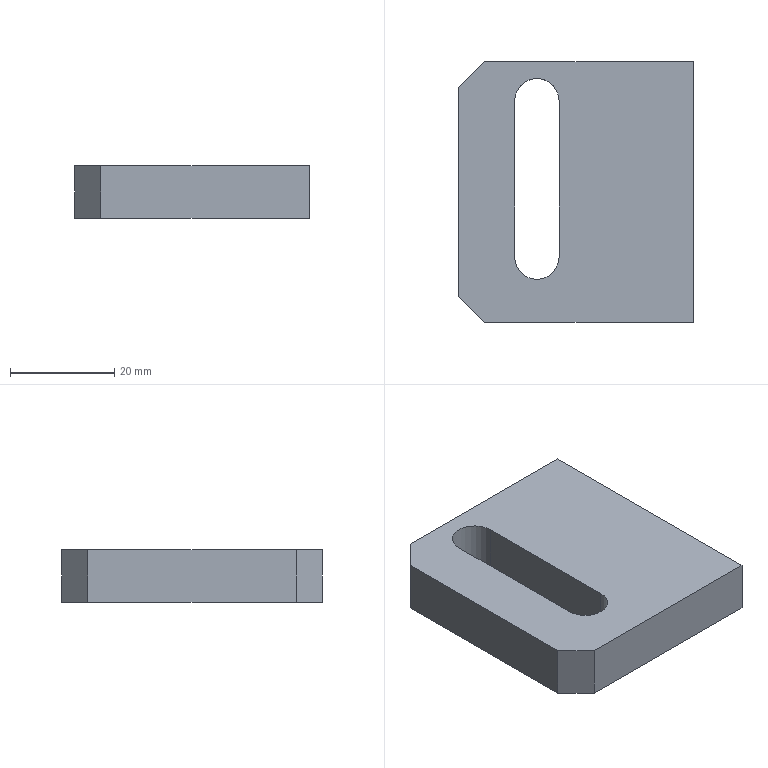Part | SolidWorks | features Chamfer 1, Extrusion 1, HoleWzd 1, ICE 1 | 1 solid | 20 faces | box 45 x 50 x 10 mm | volume 18367 mm3 | plane 10 | cylinder 6 | cone 4 | commonest cylinder face diameters 5 x4 8.5 x2
STEP:
#1=CARTESIAN_POINT('',(-6.787,32.842,7.5));
#2=VERTEX_POINT('',#1);
#3=CARTESIAN_POINT('',(-6.787,32.842,2.5));
#4=VERTEX_POINT('',#3);
#5=CARTESIAN_POINT('',(-6.787,32.842,5.));
#6=DIRECTION('',(1.,0.,0.));
#7=DIRECTION('',(0.,0.,-1.));
#8=AXIS2_PLACEMENT_3D('',#5,#6,#7);
#9=CIRCLE('',#8,2.5);
#10=EDGE_CURVE('',#2,#4,#9,.T.);
#11=ORIENTED_EDGE('',*,*,#10,.F.);
#12=CARTESIAN_POINT('',(12.213,32.842,7.5));
#13=VERTEX_POINT('',#12);
#14=CARTESIAN_POINT('',(12.213,32.842,7.5));
#15=DIRECTION('',(1.,0.,0.));
#16=VECTOR('',#15,1000.);
#17=LINE('',#14,#16);
#18=EDGE_CURVE('',#2,#13,#17,.T.);
#19=ORIENTED_EDGE('',*,*,#18,.T.);
#20=CARTESIAN_POINT('',(12.213,32.842,2.5));
#21=VERTEX_POINT('',#20);
#22=CARTESIAN_POINT('',(12.213,32.842,5.));
#23=DIRECTION('',(1.,0.,0.));
#24=DIRECTION('',(0.,0.,-1.));
#25=AXIS2_PLACEMENT_3D('',#22,#23,#24);
#26=CIRCLE('',#25,2.5);
#27=EDGE_CURVE('',#13,#21,#26,.T.);
#28=ORIENTED_EDGE('',*,*,#27,.T.);
#29=CARTESIAN_POINT('',(12.213,32.842,2.5));
#30=DIRECTION('',(1.,0.,0.));
#31=VECTOR('',#30,1000.);
#32=LINE('',#29,#31);
#33=EDGE_CURVE('',#4,#21,#32,.T.);
#34=ORIENTED_EDGE('',*,*,#33,.F.);
#35=EDGE_LOOP('',(#11,#19,#28,#34));
#36=FACE_OUTER_BOUND('',#35,.T.);
#37=CARTESIAN_POINT('',(12.213,32.842,5.));
#38=DIRECTION('',(1.,0.,0.));
#39=DIRECTION('',(0.,0.,-1.));
#40=AXIS2_PLACEMENT_3D('',#37,#38,#39);
#41=CYLINDRICAL_SURFACE('',#40,2.5);
#42=ADVANCED_FACE('',(#36),#41,.F.);
#43=CARTESIAN_POINT('',(-8.289,32.842,5.));
#44=VERTEX_POINT('',#43);
#45=CARTESIAN_POINT('',(-6.787,32.842,2.5));
#46=DIRECTION('',(0.515,0.,-0.8572));
#47=VECTOR('',#46,1000.);
#48=LINE('',#45,#47);
#49=EDGE_CURVE('',#44,#4,#48,.T.);
#50=ORIENTED_EDGE('',*,*,#49,.F.);
#51=CARTESIAN_POINT('',(-6.787,32.842,7.5));
#52=DIRECTION('',(0.515,0.,0.8572));
#53=VECTOR('',#52,1000.);
#54=LINE('',#51,#53);
#55=EDGE_CURVE('',#44,#2,#54,.T.);
#56=ORIENTED_EDGE('',*,*,#55,.T.);
#57=ORIENTED_EDGE('',*,*,#10,.T.);
#58=EDGE_LOOP('',(#50,#56,#57));
#59=FACE_OUTER_BOUND('',#58,.T.);
#60=CARTESIAN_POINT('',(-6.787,32.842,5.));
#61=DIRECTION('',(1.,0.,0.));
#62=DIRECTION('',(0.,0.,-1.));
#63=AXIS2_PLACEMENT_3D('',#60,#61,#62);
#64=CONICAL_SURFACE('',#63,2.5,1.03);
#65=ADVANCED_FACE('',(#59),#64,.F.);
#66=CARTESIAN_POINT('',(-6.787,2.842,7.5));
#67=VERTEX_POINT('',#66);
#68=CARTESIAN_POINT('',(-6.787,2.842,2.5));
#69=VERTEX_POINT('',#68);
#70=CARTESIAN_POINT('',(-6.787,2.842,5.));
#71=DIRECTION('',(1.,0.,0.));
#72=DIRECTION('',(0.,0.,-1.));
#73=AXIS2_PLACEMENT_3D('',#70,#71,#72);
#74=CIRCLE('',#73,2.5);
#75=EDGE_CURVE('',#67,#69,#74,.T.);
#76=ORIENTED_EDGE('',*,*,#75,.F.);
#77=CARTESIAN_POINT('',(12.213,2.842,7.5));
#78=VERTEX_POINT('',#77);
#79=CARTESIAN_POINT('',(12.213,2.842,7.5));
#80=DIRECTION('',(1.,0.,0.));
#81=VECTOR('',#80,1000.);
#82=LINE('',#79,#81);
#83=EDGE_CURVE('',#67,#78,#82,.T.);
#84=ORIENTED_EDGE('',*,*,#83,.T.);
#85=CARTESIAN_POINT('',(12.213,2.842,2.5));
#86=VERTEX_POINT('',#85);
#87=CARTESIAN_POINT('',(12.213,2.842,5.));
#88=DIRECTION('',(1.,0.,0.));
#89=DIRECTION('',(0.,0.,-1.));
#90=AXIS2_PLACEMENT_3D('',#87,#88,#89);
#91=CIRCLE('',#90,2.5);
#92=EDGE_CURVE('',#78,#86,#91,.T.);
#93=ORIENTED_EDGE('',*,*,#92,.T.);
#94=CARTESIAN_POINT('',(12.213,2.842,2.5));
#95=DIRECTION('',(1.,0.,0.));
#96=VECTOR('',#95,1000.);
#97=LINE('',#94,#96);
#98=EDGE_CURVE('',#69,#86,#97,.T.);
#99=ORIENTED_EDGE('',*,*,#98,.F.);
#100=EDGE_LOOP('',(#76,#84,#93,#99));
#101=FACE_OUTER_BOUND('',#100,.T.);
#102=CARTESIAN_POINT('',(12.213,2.842,5.));
#103=DIRECTION('',(1.,0.,0.));
#104=DIRECTION('',(0.,0.,-1.));
#105=AXIS2_PLACEMENT_3D('',#102,#103,#104);
#106=CYLINDRICAL_SURFACE('',#105,2.5);
#107=ADVANCED_FACE('',(#101),#106,.F.);
#108=CARTESIAN_POINT('',(-8.289,2.842,5.));
#109=VERTEX_POINT('',#108);
#110=CARTESIAN_POINT('',(-6.787,2.842,2.5));
#111=DIRECTION('',(0.515,0.,-0.8572));
#112=VECTOR('',#111,1000.);
#113=LINE('',#110,#112);
#114=EDGE_CURVE('',#109,#69,#113,.T.);
#115=ORIENTED_EDGE('',*,*,#114,.F.);
#116=CARTESIAN_POINT('',(-6.787,2.842,7.5));
#117=DIRECTION('',(0.515,0.,0.8572));
#118=VECTOR('',#117,1000.);
#119=LINE('',#116,#118);
#120=EDGE_CURVE('',#109,#67,#119,.T.);
#121=ORIENTED_EDGE('',*,*,#120,.T.);
#122=ORIENTED_EDGE('',*,*,#75,.T.);
#123=EDGE_LOOP('',(#115,#121,#122));
#124=FACE_OUTER_BOUND('',#123,.T.);
#125=CARTESIAN_POINT('',(-6.787,2.842,5.));
#126=DIRECTION('',(1.,0.,0.));
#127=DIRECTION('',(0.,0.,-1.));
#128=AXIS2_PLACEMENT_3D('',#125,#126,#127);
#129=CONICAL_SURFACE('',#128,2.5,1.03);
#130=ADVANCED_FACE('',(#124),#129,.F.);
#131=CARTESIAN_POINT('',(-32.787,42.842,10.));
#132=VERTEX_POINT('',#131);
#133=CARTESIAN_POINT('',(-32.787,2.842,10.));
#134=VERTEX_POINT('',#133);
#135=CARTESIAN_POINT('',(-32.787,47.842,10.));
#136=DIRECTION('',(0.,-1.,0.));
#137=VECTOR('',#136,1000.);
#138=LINE('',#135,#137);
#139=EDGE_CURVE('',#132,#134,#138,.T.);
#140=ORIENTED_EDGE('',*,*,#139,.F.);
#141=CARTESIAN_POINT('',(-32.787,42.842,0.));
#142=VERTEX_POINT('',#141);
#143=CARTESIAN_POINT('',(-32.787,42.842,10.));
#144=DIRECTION('',(0.,0.,-1.));
#145=VECTOR('',#144,1000.);
#146=LINE('',#143,#145);
#147=EDGE_CURVE('',#132,#142,#146,.T.);
#148=ORIENTED_EDGE('',*,*,#147,.T.);
#149=CARTESIAN_POINT('',(-32.787,2.842,0.));
#150=VERTEX_POINT('',#149);
#151=CARTESIAN_POINT('',(-32.787,47.842,0.));
#152=DIRECTION('',(0.,-1.,0.));
#153=VECTOR('',#152,1000.);
#154=LINE('',#151,#153);
#155=EDGE_CURVE('',#142,#150,#154,.T.);
#156=ORIENTED_EDGE('',*,*,#155,.T.);
#157=CARTESIAN_POINT('',(-32.787,2.842,10.));
#158=DIRECTION('',(0.,0.,1.));
#159=VECTOR('',#158,1000.);
#160=LINE('',#157,#159);
#161=EDGE_CURVE('',#150,#134,#160,.T.);
#162=ORIENTED_EDGE('',*,*,#161,.T.);
#163=EDGE_LOOP('',(#140,#148,#156,#162));
#164=FACE_OUTER_BOUND('',#163,.T.);
#165=CARTESIAN_POINT('',(-32.787,47.842,10.));
#166=DIRECTION('',(1.,0.,0.));
#167=DIRECTION('',(0.,1.,0.));
#168=AXIS2_PLACEMENT_3D('',#165,#166,#167);
#169=PLANE('',#168);
#170=ADVANCED_FACE('',(#164),#169,.F.);
#171=CARTESIAN_POINT('',(-27.787,-2.158,10.));
#172=VERTEX_POINT('',#171);
#173=CARTESIAN_POINT('',(12.213,-2.158,10.));
#174=VERTEX_POINT('',#173);
#175=CARTESIAN_POINT('',(-32.787,-2.158,10.));
#176=DIRECTION('',(1.,0.,0.));
#177=VECTOR('',#176,1000.);
#178=LINE('',#175,#177);
#179=EDGE_CURVE('',#172,#174,#178,.T.);
#180=ORIENTED_EDGE('',*,*,#179,.F.);
#181=CARTESIAN_POINT('',(-27.787,-2.158,0.));
#182=VERTEX_POINT('',#181);
#183=CARTESIAN_POINT('',(-27.787,-2.158,10.));
#184=DIRECTION('',(0.,0.,-1.));
#185=VECTOR('',#184,1000.);
#186=LINE('',#183,#185);
#187=EDGE_CURVE('',#172,#182,#186,.T.);
#188=ORIENTED_EDGE('',*,*,#187,.T.);
#189=CARTESIAN_POINT('',(12.213,-2.158,0.));
#190=VERTEX_POINT('',#189);
#191=CARTESIAN_POINT('',(-32.787,-2.158,0.));
#192=DIRECTION('',(1.,0.,0.));
#193=VECTOR('',#192,1000.);
#194=LINE('',#191,#193);
#195=EDGE_CURVE('',#182,#190,#194,.T.);
#196=ORIENTED_EDGE('',*,*,#195,.T.);
#197=CARTESIAN_POINT('',(12.213,-2.158,10.));
#198=DIRECTION('',(0.,0.,-1.));
#199=VECTOR('',#198,1000.);
#200=LINE('',#197,#199);
#201=EDGE_CURVE('',#174,#190,#200,.T.);
#202=ORIENTED_EDGE('',*,*,#201,.F.);
#203=EDGE_LOOP('',(#180,#188,#196,#202));
#204=FACE_OUTER_BOUND('',#203,.T.);
#205=CARTESIAN_POINT('',(-32.787,-2.158,10.));
#206=DIRECTION('',(0.,1.,0.));
#207=DIRECTION('',(0.,0.,1.));
#208=AXIS2_PLACEMENT_3D('',#205,#206,#207);
#209=PLANE('',#208);
#210=ADVANCED_FACE('',(#204),#209,.F.);
#211=CARTESIAN_POINT('',(12.213,32.842,5.));
#212=DIRECTION('',(1.,0.,0.));
#213=DIRECTION('',(0.,0.,-1.));
#214=AXIS2_PLACEMENT_3D('',#211,#212,#213);
#215=CIRCLE('',#214,2.5);
#216=EDGE_CURVE('',#21,#13,#215,.T.);
#217=ORIENTED_EDGE('',*,*,#216,.F.);
#218=ORIENTED_EDGE('',*,*,#27,.F.);
#219=EDGE_LOOP('',(#217,#218));
#220=FACE_BOUND('',#219,.T.);
#221=CARTESIAN_POINT('',(12.213,2.842,5.));
#222=DIRECTION('',(1.,0.,0.));
#223=DIRECTION('',(0.,0.,-1.));
#224=AXIS2_PLACEMENT_3D('',#221,#222,#223);
#225=CIRCLE('',#224,2.5);
#226=EDGE_CURVE('',#86,#78,#225,.T.);
#227=ORIENTED_EDGE('',*,*,#226,.F.);
#228=ORIENTED_EDGE('',*,*,#92,.F.);
#229=EDGE_LOOP('',(#227,#228));
#230=FACE_BOUND('',#229,.T.);
#231=CARTESIAN_POINT('',(12.213,47.842,0.));
#232=VERTEX_POINT('',#231);
#233=CARTESIAN_POINT('',(12.213,47.842,0.));
#234=DIRECTION('',(0.,1.,0.));
#235=VECTOR('',#234,1000.);
#236=LINE('',#233,#235);
#237=EDGE_CURVE('',#190,#232,#236,.T.);
#238=ORIENTED_EDGE('',*,*,#237,.T.);
#239=CARTESIAN_POINT('',(12.213,47.842,10.));
#240=VERTEX_POINT('',#239);
#241=CARTESIAN_POINT('',(12.213,47.842,10.));
#242=DIRECTION('',(0.,0.,-1.));
#243=VECTOR('',#242,1000.);
#244=LINE('',#241,#243);
#245=EDGE_CURVE('',#240,#232,#244,.T.);
#246=ORIENTED_EDGE('',*,*,#245,.F.);
#247=CARTESIAN_POINT('',(12.213,47.842,10.));
#248=DIRECTION('',(0.,1.,0.));
#249=VECTOR('',#248,1000.);
#250=LINE('',#247,#249);
#251=EDGE_CURVE('',#174,#240,#250,.T.);
#252=ORIENTED_EDGE('',*,*,#251,.F.);
#253=ORIENTED_EDGE('',*,*,#201,.T.);
#254=EDGE_LOOP('',(#238,#246,#252,#253));
#255=FACE_OUTER_BOUND('',#254,.T.);
#256=CARTESIAN_POINT('',(12.213,47.842,10.));
#257=DIRECTION('',(-1.,0.,0.));
#258=DIRECTION('',(0.,-1.,0.));
#259=AXIS2_PLACEMENT_3D('',#256,#257,#258);
#260=PLANE('',#259);
#261=ADVANCED_FACE('',(#220,#230,#255),#260,.F.);
#262=CARTESIAN_POINT('',(-27.787,47.842,0.));
#263=VERTEX_POINT('',#262);
#264=CARTESIAN_POINT('',(-32.787,47.842,0.));
#265=DIRECTION('',(-1.,0.,0.));
#266=VECTOR('',#265,1000.);
#267=LINE('',#264,#266);
#268=EDGE_CURVE('',#232,#263,#267,.T.);
#269=ORIENTED_EDGE('',*,*,#268,.T.);
#270=CARTESIAN_POINT('',(-27.787,47.842,10.));
#271=VERTEX_POINT('',#270);
#272=CARTESIAN_POINT('',(-27.787,47.842,10.));
#273=DIRECTION('',(0.,0.,1.));
#274=VECTOR('',#273,1000.);
#275=LINE('',#272,#274);
#276=EDGE_CURVE('',#263,#271,#275,.T.);
#277=ORIENTED_EDGE('',*,*,#276,.T.);
#278=CARTESIAN_POINT('',(-32.787,47.842,10.));
#279=DIRECTION('',(-1.,0.,0.));
#280=VECTOR('',#279,1000.);
#281=LINE('',#278,#280);
#282=EDGE_CURVE('',#240,#271,#281,.T.);
#283=ORIENTED_EDGE('',*,*,#282,.F.);
#284=ORIENTED_EDGE('',*,*,#245,.T.);
#285=EDGE_LOOP('',(#269,#277,#283,#284));
#286=FACE_OUTER_BOUND('',#285,.T.);
#287=CARTESIAN_POINT('',(-32.787,47.842,10.));
#288=DIRECTION('',(0.,-1.,0.));
#289=DIRECTION('',(0.,0.,-1.));
#290=AXIS2_PLACEMENT_3D('',#287,#288,#289);
#291=PLANE('',#290);
#292=ADVANCED_FACE('',(#286),#291,.F.);
#293=CARTESIAN_POINT('',(-13.537,40.342,10.));
#294=VERTEX_POINT('',#293);
#295=CARTESIAN_POINT('',(-22.037,40.342,10.));
#296=VERTEX_POINT('',#295);
#297=CARTESIAN_POINT('',(-17.787,40.342,10.));
#298=DIRECTION('',(0.,0.,1.));
#299=DIRECTION('',(1.,0.,0.));
#300=AXIS2_PLACEMENT_3D('',#297,#298,#299);
#301=CIRCLE('',#300,4.25);
#302=EDGE_CURVE('',#294,#296,#301,.T.);
#303=ORIENTED_EDGE('',*,*,#302,.F.);
#304=CARTESIAN_POINT('',(-13.537,10.342,10.));
#305=VERTEX_POINT('',#304);
#306=CARTESIAN_POINT('',(-13.537,40.342,10.));
#307=DIRECTION('',(0.,1.,0.));
#308=VECTOR('',#307,1000.);
#309=LINE('',#306,#308);
#310=EDGE_CURVE('',#305,#294,#309,.T.);
#311=ORIENTED_EDGE('',*,*,#310,.F.);
#312=CARTESIAN_POINT('',(-22.037,10.342,10.));
#313=VERTEX_POINT('',#312);
#314=CARTESIAN_POINT('',(-17.787,10.342,10.));
#315=DIRECTION('',(0.,0.,1.));
#316=DIRECTION('',(1.,0.,0.));
#317=AXIS2_PLACEMENT_3D('',#314,#315,#316);
#318=CIRCLE('',#317,4.25);
#319=EDGE_CURVE('',#313,#305,#318,.T.);
#320=ORIENTED_EDGE('',*,*,#319,.F.);
#321=CARTESIAN_POINT('',(-22.037,40.342,10.));
#322=DIRECTION('',(0.,-1.,0.));
#323=VECTOR('',#322,1000.);
#324=LINE('',#321,#323);
#325=EDGE_CURVE('',#296,#313,#324,.T.);
#326=ORIENTED_EDGE('',*,*,#325,.F.);
#327=EDGE_LOOP('',(#303,#311,#320,#326));
#328=FACE_BOUND('',#327,.T.);
#329=ORIENTED_EDGE('',*,*,#282,.T.);
#330=CARTESIAN_POINT('',(-37.815,37.815,10.));
#331=DIRECTION('',(-0.7071,-0.7071,0.));
#332=VECTOR('',#331,1000.);
#333=LINE('',#330,#332);
#334=EDGE_CURVE('',#271,#132,#333,.T.);
#335=ORIENTED_EDGE('',*,*,#334,.T.);
#336=ORIENTED_EDGE('',*,*,#139,.T.);
#337=CARTESIAN_POINT('',(-14.972,-14.972,10.));
#338=DIRECTION('',(0.7071,-0.7071,0.));
#339=VECTOR('',#338,1000.);
#340=LINE('',#337,#339);
#341=EDGE_CURVE('',#134,#172,#340,.T.);
#342=ORIENTED_EDGE('',*,*,#341,.T.);
#343=ORIENTED_EDGE('',*,*,#179,.T.);
#344=ORIENTED_EDGE('',*,*,#251,.T.);
#345=EDGE_LOOP('',(#329,#335,#336,#342,#343,#344));
#346=FACE_OUTER_BOUND('',#345,.T.);
#347=CARTESIAN_POINT('',(0.,0.,10.));
#348=DIRECTION('',(0.,0.,1.));
#349=DIRECTION('',(1.,0.,0.));
#350=AXIS2_PLACEMENT_3D('',#347,#348,#349);
#351=PLANE('',#350);
#352=ADVANCED_FACE('',(#328,#346),#351,.T.);
#353=CARTESIAN_POINT('',(-13.537,10.342,0.));
#354=VERTEX_POINT('',#353);
#355=CARTESIAN_POINT('',(-13.537,40.342,0.));
#356=VERTEX_POINT('',#355);
#357=CARTESIAN_POINT('',(-13.537,40.342,0.));
#358=DIRECTION('',(0.,1.,0.));
#359=VECTOR('',#358,1000.);
#360=LINE('',#357,#359);
#361=EDGE_CURVE('',#354,#356,#360,.T.);
#362=ORIENTED_EDGE('',*,*,#361,.T.);
#363=CARTESIAN_POINT('',(-22.037,40.342,0.));
#364=VERTEX_POINT('',#363);
#365=CARTESIAN_POINT('',(-17.787,40.342,0.));
#366=DIRECTION('',(0.,0.,1.));
#367=DIRECTION('',(1.,0.,0.));
#368=AXIS2_PLACEMENT_3D('',#365,#366,#367);
#369=CIRCLE('',#368,4.25);
#370=EDGE_CURVE('',#356,#364,#369,.T.);
#371=ORIENTED_EDGE('',*,*,#370,.T.);
#372=CARTESIAN_POINT('',(-22.037,10.342,0.));
#373=VERTEX_POINT('',#372);
#374=CARTESIAN_POINT('',(-22.037,40.342,0.));
#375=DIRECTION('',(0.,-1.,0.));
#376=VECTOR('',#375,1000.);
#377=LINE('',#374,#376);
#378=EDGE_CURVE('',#364,#373,#377,.T.);
#379=ORIENTED_EDGE('',*,*,#378,.T.);
#380=CARTESIAN_POINT('',(-17.787,10.342,0.));
#381=DIRECTION('',(0.,0.,1.));
#382=DIRECTION('',(1.,0.,0.));
#383=AXIS2_PLACEMENT_3D('',#380,#381,#382);
#384=CIRCLE('',#383,4.25);
#385=EDGE_CURVE('',#373,#354,#384,.T.);
#386=ORIENTED_EDGE('',*,*,#385,.T.);
#387=EDGE_LOOP('',(#362,#371,#379,#386));
#388=FACE_BOUND('',#387,.T.);
#389=ORIENTED_EDGE('',*,*,#155,.F.);
#390=CARTESIAN_POINT('',(-32.787,42.842,0.));
#391=DIRECTION('',(0.7071,0.7071,0.));
#392=VECTOR('',#391,1000.);
#393=LINE('',#390,#392);
#394=EDGE_CURVE('',#142,#263,#393,.T.);
#395=ORIENTED_EDGE('',*,*,#394,.T.);
#396=ORIENTED_EDGE('',*,*,#268,.F.);
#397=ORIENTED_EDGE('',*,*,#237,.F.);
#398=ORIENTED_EDGE('',*,*,#195,.F.);
#399=CARTESIAN_POINT('',(-27.787,-2.158,0.));
#400=DIRECTION('',(-0.7071,0.7071,0.));
#401=VECTOR('',#400,1000.);
#402=LINE('',#399,#401);
#403=EDGE_CURVE('',#182,#150,#402,.T.);
#404=ORIENTED_EDGE('',*,*,#403,.T.);
#405=EDGE_LOOP('',(#389,#395,#396,#397,#398,#404));
#406=FACE_OUTER_BOUND('',#405,.T.);
#407=CARTESIAN_POINT('',(0.,0.,0.));
#408=DIRECTION('',(0.,0.,1.));
#409=DIRECTION('',(1.,0.,0.));
#410=AXIS2_PLACEMENT_3D('',#407,#408,#409);
#411=PLANE('',#410);
#412=ADVANCED_FACE('',(#388,#406),#411,.F.);
#413=ORIENTED_EDGE('',*,*,#302,.T.);
#414=CARTESIAN_POINT('',(-22.037,40.342,0.));
#415=DIRECTION('',(0.,0.,1.));
#416=VECTOR('',#415,1000.);
#417=LINE('',#414,#416);
#418=EDGE_CURVE('',#364,#296,#417,.T.);
#419=ORIENTED_EDGE('',*,*,#418,.F.);
#420=ORIENTED_EDGE('',*,*,#370,.F.);
#421=CARTESIAN_POINT('',(-13.537,40.342,0.));
#422=DIRECTION('',(0.,0.,1.));
#423=VECTOR('',#422,1000.);
#424=LINE('',#421,#423);
#425=EDGE_CURVE('',#356,#294,#424,.T.);
#426=ORIENTED_EDGE('',*,*,#425,.T.);
#427=EDGE_LOOP('',(#413,#419,#420,#426));
#428=FACE_OUTER_BOUND('',#427,.T.);
#429=CARTESIAN_POINT('',(-17.787,40.342,0.));
#430=DIRECTION('',(0.,0.,1.));
#431=DIRECTION('',(1.,0.,0.));
#432=AXIS2_PLACEMENT_3D('',#429,#430,#431);
#433=CYLINDRICAL_SURFACE('',#432,4.25);
#434=ADVANCED_FACE('',(#428),#433,.F.);
#435=ORIENTED_EDGE('',*,*,#310,.T.);
#436=ORIENTED_EDGE('',*,*,#425,.F.);
#437=ORIENTED_EDGE('',*,*,#361,.F.);
#438=CARTESIAN_POINT('',(-13.537,10.342,0.));
#439=DIRECTION('',(0.,0.,1.));
#440=VECTOR('',#439,1000.);
#441=LINE('',#438,#440);
#442=EDGE_CURVE('',#354,#305,#441,.T.);
#443=ORIENTED_EDGE('',*,*,#442,.T.);
#444=EDGE_LOOP('',(#435,#436,#437,#443));
#445=FACE_OUTER_BOUND('',#444,.T.);
#446=CARTESIAN_POINT('',(-13.537,40.342,0.));
#447=DIRECTION('',(1.,0.,0.));
#448=DIRECTION('',(0.,1.,0.));
#449=AXIS2_PLACEMENT_3D('',#446,#447,#448);
#450=PLANE('',#449);
#451=ADVANCED_FACE('',(#445),#450,.F.);
#452=ORIENTED_EDGE('',*,*,#319,.T.);
#453=ORIENTED_EDGE('',*,*,#442,.F.);
#454=ORIENTED_EDGE('',*,*,#385,.F.);
#455=CARTESIAN_POINT('',(-22.037,10.342,0.));
#456=DIRECTION('',(0.,0.,1.));
#457=VECTOR('',#456,1000.);
#458=LINE('',#455,#457);
#459=EDGE_CURVE('',#373,#313,#458,.T.);
#460=ORIENTED_EDGE('',*,*,#459,.T.);
#461=EDGE_LOOP('',(#452,#453,#454,#460));
#462=FACE_OUTER_BOUND('',#461,.T.);
#463=CARTESIAN_POINT('',(-17.787,10.342,0.));
#464=DIRECTION('',(0.,0.,1.));
#465=DIRECTION('',(1.,0.,0.));
#466=AXIS2_PLACEMENT_3D('',#463,#464,#465);
#467=CYLINDRICAL_SURFACE('',#466,4.25);
#468=ADVANCED_FACE('',(#462),#467,.F.);
#469=ORIENTED_EDGE('',*,*,#325,.T.);
#470=ORIENTED_EDGE('',*,*,#459,.F.);
#471=ORIENTED_EDGE('',*,*,#378,.F.);
#472=ORIENTED_EDGE('',*,*,#418,.T.);
#473=EDGE_LOOP('',(#469,#470,#471,#472));
#474=FACE_OUTER_BOUND('',#473,.T.);
#475=CARTESIAN_POINT('',(-22.037,40.342,0.));
#476=DIRECTION('',(-1.,0.,0.));
#477=DIRECTION('',(0.,0.,1.));
#478=AXIS2_PLACEMENT_3D('',#475,#476,#477);
#479=PLANE('',#478);
#480=ADVANCED_FACE('',(#474),#479,.F.);
#481=ORIENTED_EDGE('',*,*,#334,.F.);
#482=ORIENTED_EDGE('',*,*,#276,.F.);
#483=ORIENTED_EDGE('',*,*,#394,.F.);
#484=ORIENTED_EDGE('',*,*,#147,.F.);
#485=EDGE_LOOP('',(#481,#482,#483,#484));
#486=FACE_OUTER_BOUND('',#485,.T.);
#487=CARTESIAN_POINT('',(-32.787,42.842,10.));
#488=DIRECTION('',(0.7071,-0.7071,0.));
#489=DIRECTION('',(0.,0.,-1.));
#490=AXIS2_PLACEMENT_3D('',#487,#488,#489);
#491=PLANE('',#490);
#492=ADVANCED_FACE('',(#486),#491,.F.);
#493=ORIENTED_EDGE('',*,*,#341,.F.);
#494=ORIENTED_EDGE('',*,*,#161,.F.);
#495=ORIENTED_EDGE('',*,*,#403,.F.);
#496=ORIENTED_EDGE('',*,*,#187,.F.);
#497=EDGE_LOOP('',(#493,#494,#495,#496));
#498=FACE_OUTER_BOUND('',#497,.T.);
#499=CARTESIAN_POINT('',(-27.787,-2.158,10.));
#500=DIRECTION('',(0.7071,0.7071,0.));
#501=DIRECTION('',(0.,0.,-1.));
#502=AXIS2_PLACEMENT_3D('',#499,#500,#501);
#503=PLANE('',#502);
#504=ADVANCED_FACE('',(#498),#503,.F.);
#505=ORIENTED_EDGE('',*,*,#120,.F.);
#506=ORIENTED_EDGE('',*,*,#114,.T.);
#507=CARTESIAN_POINT('',(-6.787,2.842,5.));
#508=DIRECTION('',(1.,0.,0.));
#509=DIRECTION('',(0.,0.,-1.));
#510=AXIS2_PLACEMENT_3D('',#507,#508,#509);
#511=CIRCLE('',#510,2.5);
#512=EDGE_CURVE('',#69,#67,#511,.T.);
#513=ORIENTED_EDGE('',*,*,#512,.T.);
#514=EDGE_LOOP('',(#505,#506,#513));
#515=FACE_OUTER_BOUND('',#514,.T.);
#516=CARTESIAN_POINT('',(-6.787,2.842,5.));
#517=DIRECTION('',(1.,0.,0.));
#518=DIRECTION('',(0.,0.,-1.));
#519=AXIS2_PLACEMENT_3D('',#516,#517,#518);
#520=CONICAL_SURFACE('',#519,2.5,1.03);
#521=ADVANCED_FACE('',(#515),#520,.F.);
#522=ORIENTED_EDGE('',*,*,#83,.F.);
#523=ORIENTED_EDGE('',*,*,#512,.F.);
#524=ORIENTED_EDGE('',*,*,#98,.T.);
#525=ORIENTED_EDGE('',*,*,#226,.T.);
#526=EDGE_LOOP('',(#522,#523,#524,#525));
#527=FACE_OUTER_BOUND('',#526,.T.);
#528=CARTESIAN_POINT('',(12.213,2.842,5.));
#529=DIRECTION('',(1.,0.,0.));
#530=DIRECTION('',(0.,0.,-1.));
#531=AXIS2_PLACEMENT_3D('',#528,#529,#530);
#532=CYLINDRICAL_SURFACE('',#531,2.5);
#533=ADVANCED_FACE('',(#527),#532,.F.);
#534=ORIENTED_EDGE('',*,*,#55,.F.);
#535=ORIENTED_EDGE('',*,*,#49,.T.);
#536=CARTESIAN_POINT('',(-6.787,32.842,5.));
#537=DIRECTION('',(1.,0.,0.));
#538=DIRECTION('',(0.,0.,-1.));
#539=AXIS2_PLACEMENT_3D('',#536,#537,#538);
#540=CIRCLE('',#539,2.5);
#541=EDGE_CURVE('',#4,#2,#540,.T.);
#542=ORIENTED_EDGE('',*,*,#541,.T.);
#543=EDGE_LOOP('',(#534,#535,#542));
#544=FACE_OUTER_BOUND('',#543,.T.);
#545=CARTESIAN_POINT('',(-6.787,32.842,5.));
#546=DIRECTION('',(1.,0.,0.));
#547=DIRECTION('',(0.,0.,-1.));
#548=AXIS2_PLACEMENT_3D('',#545,#546,#547);
#549=CONICAL_SURFACE('',#548,2.5,1.03);
#550=ADVANCED_FACE('',(#544),#549,.F.);
#551=ORIENTED_EDGE('',*,*,#18,.F.);
#552=ORIENTED_EDGE('',*,*,#541,.F.);
#553=ORIENTED_EDGE('',*,*,#33,.T.);
#554=ORIENTED_EDGE('',*,*,#216,.T.);
#555=EDGE_LOOP('',(#551,#552,#553,#554));
#556=FACE_OUTER_BOUND('',#555,.T.);
#557=CARTESIAN_POINT('',(12.213,32.842,5.));
#558=DIRECTION('',(1.,0.,0.));
#559=DIRECTION('',(0.,0.,-1.));
#560=AXIS2_PLACEMENT_3D('',#557,#558,#559);
#561=CYLINDRICAL_SURFACE('',#560,2.5);
#562=ADVANCED_FACE('',(#556),#561,.F.);
#563=CLOSED_SHELL('',(#42,#65,#107,#130,#170,#210,#261,#292,#352,#412,#434,#451,#468,#480,#492,#504,#521,#533,#550,#562));
#564=MANIFOLD_SOLID_BREP('',#563);
#565=CARTESIAN_POINT('',(0.,0.,0.));
#566=DIRECTION('',(0.,0.,1.));
#567=DIRECTION('',(1.,0.,0.));
#568=AXIS2_PLACEMENT_3D('',#565,#566,#567);
#569=(LENGTH_UNIT()NAMED_UNIT(*)SI_UNIT(.MILLI.,.METRE.));
#570=UNCERTAINTY_MEASURE_WITH_UNIT(LENGTH_MEASURE(0.00001),#569,'','');
#571=(NAMED_UNIT(*)PLANE_ANGLE_UNIT()SI_UNIT($,.RADIAN.));
#572=(NAMED_UNIT(*)SI_UNIT($,.STERADIAN.)SOLID_ANGLE_UNIT());
#573=(GEOMETRIC_REPRESENTATION_CONTEXT(3)GLOBAL_UNCERTAINTY_ASSIGNED_CONTEXT((#570))GLOBAL_UNIT_ASSIGNED_CONTEXT((#569,#571,#572))REPRESENTATION_CONTEXT('',''));
#574=ADVANCED_BREP_SHAPE_REPRESENTATION('',(#564,#568),#573);